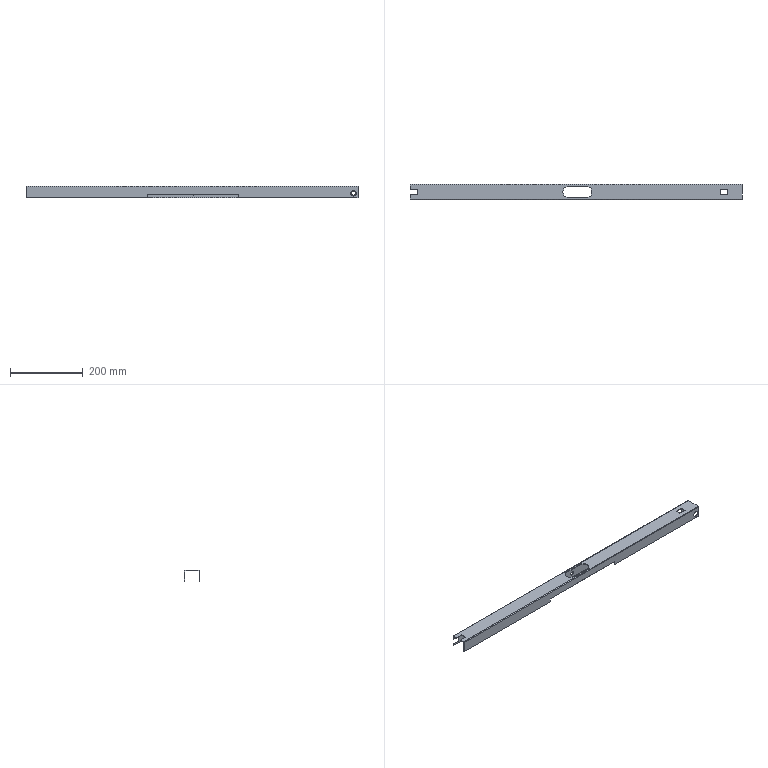Part | 1 solid | 68 faces | box 912 x 42 x 32 mm | volume 128731 mm3 | plane 48 | cylinder 20 | commonest cylinder face diameters 10 x10 0.4 x2 3.4 x2 11 x2 15 x2 30 x2